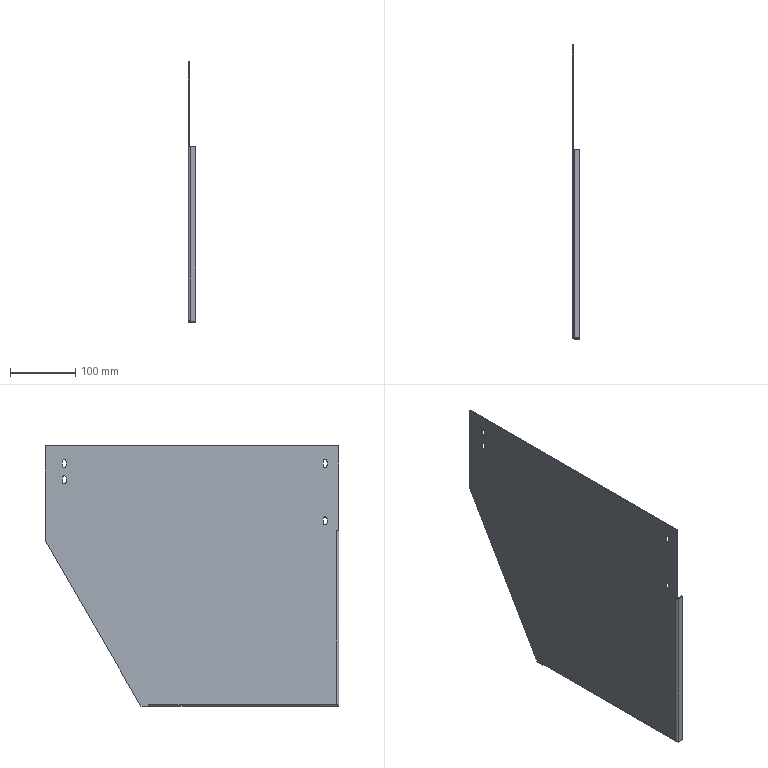Part | NX | features solid 2 | 1 solid | 50 faces | box 12 x 450 x 399 mm | volume 248985 mm3 | plane 38 | cylinder 12 | commonest cylinder face diameters 6 x10 3 x2
STEP:
#1=CARTESIAN_POINT('',(-1108.5,341.153,-601.));
#2=VERTEX_POINT('',#1);
#3=CARTESIAN_POINT('',(-1108.5,53.,-601.));
#4=VERTEX_POINT('',#3);
#5=CARTESIAN_POINT('',(-1108.5,341.153,-601.));
#6=DIRECTION('',(0.,-1.,0.));
#7=VECTOR('',#6,1000.);
#8=LINE('',#5,#7);
#9=EDGE_CURVE('',#2,#4,#8,.T.);
#10=ORIENTED_EDGE('',*,*,#9,.T.);
#11=CARTESIAN_POINT('',(-1107.,51.6,-602.5));
#12=VERTEX_POINT('',#11);
#13=CARTESIAN_POINT('',(-1107.,51.6,-602.5));
#14=CARTESIAN_POINT('',(-1107.879,51.6,-602.5));
#15=CARTESIAN_POINT('',(-1108.5,52.18,-601.879));
#16=CARTESIAN_POINT('',(-1108.5,53.,-601.));
#17=(BOUNDED_CURVE()B_SPLINE_CURVE(3,(#13,#14,#15,#16),.UNSPECIFIED.,.F.,.F.)B_SPLINE_CURVE_WITH_KNOTS((4,4),(0.,1.571),.PIECEWISE_BEZIER_KNOTS.)CURVE()GEOMETRIC_REPRESENTATION_ITEM()RATIONAL_B_SPLINE_CURVE((1.,0.8047,0.8047,1.))REPRESENTATION_ITEM(''));
#18=EDGE_CURVE('',#12,#4,#17,.T.);
#19=ORIENTED_EDGE('',*,*,#18,.F.);
#20=CARTESIAN_POINT('',(-1107.,341.153,-602.5));
#21=VERTEX_POINT('',#20);
#22=CARTESIAN_POINT('',(-1107.,53.,-602.5));
#23=DIRECTION('',(0.,1.,0.));
#24=VECTOR('',#23,1000.);
#25=LINE('',#22,#24);
#26=EDGE_CURVE('',#12,#21,#25,.T.);
#27=ORIENTED_EDGE('',*,*,#26,.T.);
#28=CARTESIAN_POINT('',(-1107.,341.153,-601.));
#29=DIRECTION('',(0.,1.,0.));
#30=DIRECTION('',(-1.,0.,0.));
#31=AXIS2_PLACEMENT_3D('',#28,#29,#30);
#32=CIRCLE('',#31,1.5);
#33=EDGE_CURVE('',#21,#2,#32,.T.);
#34=ORIENTED_EDGE('',*,*,#33,.T.);
#35=EDGE_LOOP('',(#10,#19,#27,#34));
#36=FACE_BOUND('',#35,.T.);
#37=CARTESIAN_POINT('',(-1107.,341.153,-601.));
#38=DIRECTION('',(0.,-1.,0.));
#39=DIRECTION('',(1.,0.,0.));
#40=AXIS2_PLACEMENT_3D('',#37,#38,#39);
#41=CYLINDRICAL_SURFACE('',#40,1.5);
#42=ADVANCED_FACE('',(#36),#41,.F.);
#43=CARTESIAN_POINT('',(-1110.,341.153,-601.));
#44=VERTEX_POINT('',#43);
#45=CARTESIAN_POINT('',(-1110.,53.,-601.));
#46=VERTEX_POINT('',#45);
#47=CARTESIAN_POINT('',(-1110.,341.153,-601.));
#48=DIRECTION('',(0.,-1.,0.));
#49=VECTOR('',#48,1000.);
#50=LINE('',#47,#49);
#51=EDGE_CURVE('',#44,#46,#50,.T.);
#52=ORIENTED_EDGE('',*,*,#51,.F.);
#53=CARTESIAN_POINT('',(-1107.,341.153,-604.));
#54=VERTEX_POINT('',#53);
#55=CARTESIAN_POINT('',(-1107.,341.153,-601.));
#56=DIRECTION('',(0.,1.,0.));
#57=DIRECTION('',(1.,0.,0.));
#58=AXIS2_PLACEMENT_3D('',#55,#56,#57);
#59=CIRCLE('',#58,3.);
#60=EDGE_CURVE('',#54,#44,#59,.T.);
#61=ORIENTED_EDGE('',*,*,#60,.F.);
#62=CARTESIAN_POINT('',(-1107.,51.6,-604.));
#63=VERTEX_POINT('',#62);
#64=CARTESIAN_POINT('',(-1107.,53.,-604.));
#65=DIRECTION('',(0.,1.,0.));
#66=VECTOR('',#65,1000.);
#67=LINE('',#64,#66);
#68=EDGE_CURVE('',#63,#54,#67,.T.);
#69=ORIENTED_EDGE('',*,*,#68,.F.);
#70=CARTESIAN_POINT('',(-1109.598,51.6,-602.5));
#71=VERTEX_POINT('',#70);
#72=CARTESIAN_POINT('',(-1107.,51.6,-601.));
#73=DIRECTION('',(0.,1.,0.));
#74=DIRECTION('',(1.,0.,0.));
#75=AXIS2_PLACEMENT_3D('',#72,#73,#74);
#76=CIRCLE('',#75,3.);
#77=EDGE_CURVE('',#63,#71,#76,.T.);
#78=ORIENTED_EDGE('',*,*,#77,.T.);
#79=CARTESIAN_POINT('',(-1109.598,51.6,-602.5));
#80=CARTESIAN_POINT('',(-1109.863,52.028,-602.041));
#81=CARTESIAN_POINT('',(-1110.,52.506,-601.53));
#82=CARTESIAN_POINT('',(-1110.,53.,-601.));
#83=(BOUNDED_CURVE()B_SPLINE_CURVE(3,(#79,#80,#81,#82),.UNSPECIFIED.,.F.,.F.)B_SPLINE_CURVE_WITH_KNOTS((4,4),(1.047,1.571),.PIECEWISE_BEZIER_KNOTS.)CURVE()GEOMETRIC_REPRESENTATION_ITEM()RATIONAL_B_SPLINE_CURVE((1.,0.9773,0.9773,1.))REPRESENTATION_ITEM(''));
#84=EDGE_CURVE('',#71,#46,#83,.T.);
#85=ORIENTED_EDGE('',*,*,#84,.T.);
#86=EDGE_LOOP('',(#52,#61,#69,#78,#85));
#87=FACE_BOUND('',#86,.T.);
#88=CARTESIAN_POINT('',(-1107.,341.153,-601.));
#89=DIRECTION('',(0.,-1.,0.));
#90=DIRECTION('',(1.,0.,0.));
#91=AXIS2_PLACEMENT_3D('',#88,#89,#90);
#92=CYLINDRICAL_SURFACE('',#91,3.);
#93=ADVANCED_FACE('',(#87),#92,.T.);
#94=CARTESIAN_POINT('',(-1098.,341.153,-602.5));
#95=VERTEX_POINT('',#94);
#96=CARTESIAN_POINT('',(-1098.,51.6,-602.5));
#97=VERTEX_POINT('',#96);
#98=CARTESIAN_POINT('',(-1098.,341.153,-602.5));
#99=DIRECTION('',(0.,-1.,0.));
#100=VECTOR('',#99,1000.);
#101=LINE('',#98,#100);
#102=EDGE_CURVE('',#95,#97,#101,.T.);
#103=ORIENTED_EDGE('',*,*,#102,.T.);
#104=CARTESIAN_POINT('',(-1098.,51.6,-604.));
#105=VERTEX_POINT('',#104);
#106=CARTESIAN_POINT('',(-1098.,51.6,-604.));
#107=DIRECTION('',(0.,0.,1.));
#108=VECTOR('',#107,1000.);
#109=LINE('',#106,#108);
#110=EDGE_CURVE('',#105,#97,#109,.T.);
#111=ORIENTED_EDGE('',*,*,#110,.F.);
#112=CARTESIAN_POINT('',(-1098.,341.153,-604.));
#113=VERTEX_POINT('',#112);
#114=CARTESIAN_POINT('',(-1098.,341.153,-604.));
#115=DIRECTION('',(0.,-1.,0.));
#116=VECTOR('',#115,1000.);
#117=LINE('',#114,#116);
#118=EDGE_CURVE('',#113,#105,#117,.T.);
#119=ORIENTED_EDGE('',*,*,#118,.F.);
#120=CARTESIAN_POINT('',(-1098.,341.153,-604.));
#121=DIRECTION('',(0.,0.,1.));
#122=VECTOR('',#121,1000.);
#123=LINE('',#120,#122);
#124=EDGE_CURVE('',#113,#95,#123,.T.);
#125=ORIENTED_EDGE('',*,*,#124,.T.);
#126=EDGE_LOOP('',(#103,#111,#119,#125));
#127=FACE_BOUND('',#126,.T.);
#128=CARTESIAN_POINT('',(-1098.,341.153,-604.));
#129=DIRECTION('',(-1.,0.,0.));
#130=DIRECTION('',(0.,0.,1.));
#131=AXIS2_PLACEMENT_3D('',#128,#129,#130);
#132=PLANE('',#131);
#133=ADVANCED_FACE('',(#127),#132,.F.);
#134=ORIENTED_EDGE('',*,*,#26,.F.);
#135=CARTESIAN_POINT('',(-1108.649,51.6,-602.5));
#136=DIRECTION('',(-1.,0.,0.));
#137=VECTOR('',#136,1000.);
#138=LINE('',#135,#137);
#139=EDGE_CURVE('',#97,#12,#138,.T.);
#140=ORIENTED_EDGE('',*,*,#139,.F.);
#141=ORIENTED_EDGE('',*,*,#102,.F.);
#142=CARTESIAN_POINT('',(-1108.649,341.153,-602.5));
#143=DIRECTION('',(1.,0.,0.));
#144=VECTOR('',#143,1000.);
#145=LINE('',#142,#144);
#146=EDGE_CURVE('',#21,#95,#145,.T.);
#147=ORIENTED_EDGE('',*,*,#146,.F.);
#148=EDGE_LOOP('',(#134,#140,#141,#147));
#149=FACE_BOUND('',#148,.T.);
#150=CARTESIAN_POINT('',(-722.5,275.,-602.5));
#151=DIRECTION('',(0.,0.,-1.));
#152=DIRECTION('',(-1.,0.,0.));
#153=AXIS2_PLACEMENT_3D('',#150,#151,#152);
#154=PLANE('',#153);
#155=ADVANCED_FACE('',(#149),#154,.F.);
#156=CARTESIAN_POINT('',(-1108.649,51.6,-604.));
#157=DIRECTION('',(-1.,0.,0.));
#158=VECTOR('',#157,1000.);
#159=LINE('',#156,#158);
#160=EDGE_CURVE('',#105,#63,#159,.T.);
#161=ORIENTED_EDGE('',*,*,#160,.T.);
#162=ORIENTED_EDGE('',*,*,#68,.T.);
#163=CARTESIAN_POINT('',(-1108.649,341.153,-604.));
#164=DIRECTION('',(1.,0.,0.));
#165=VECTOR('',#164,1000.);
#166=LINE('',#163,#165);
#167=EDGE_CURVE('',#54,#113,#166,.T.);
#168=ORIENTED_EDGE('',*,*,#167,.T.);
#169=ORIENTED_EDGE('',*,*,#118,.T.);
#170=EDGE_LOOP('',(#161,#162,#168,#169));
#171=FACE_BOUND('',#170,.T.);
#172=CARTESIAN_POINT('',(-722.5,275.,-604.));
#173=DIRECTION('',(0.,0.,-1.));
#174=DIRECTION('',(-1.,0.,0.));
#175=AXIS2_PLACEMENT_3D('',#172,#173,#174);
#176=PLANE('',#175);
#177=ADVANCED_FACE('',(#171),#176,.T.);
#178=CARTESIAN_POINT('',(-1107.,51.6,-604.));
#179=DIRECTION('',(0.,0.,1.));
#180=VECTOR('',#179,1000.);
#181=LINE('',#178,#180);
#182=EDGE_CURVE('',#63,#12,#181,.T.);
#183=ORIENTED_EDGE('',*,*,#182,.F.);
#184=ORIENTED_EDGE('',*,*,#160,.F.);
#185=ORIENTED_EDGE('',*,*,#110,.T.);
#186=ORIENTED_EDGE('',*,*,#139,.T.);
#187=EDGE_LOOP('',(#183,#184,#185,#186));
#188=FACE_BOUND('',#187,.T.);
#189=CARTESIAN_POINT('',(-1108.649,51.6,-604.));
#190=DIRECTION('',(0.,1.,0.));
#191=DIRECTION('',(0.,0.,-1.));
#192=AXIS2_PLACEMENT_3D('',#189,#190,#191);
#193=PLANE('',#192);
#194=ADVANCED_FACE('',(#188),#193,.F.);
#195=CARTESIAN_POINT('',(-1107.,50.,-602.4));
#196=VERTEX_POINT('',#195);
#197=CARTESIAN_POINT('',(-1107.,50.,-604.));
#198=VERTEX_POINT('',#197);
#199=CARTESIAN_POINT('',(-1107.,50.,-601.));
#200=DIRECTION('',(0.,0.,-1.));
#201=VECTOR('',#200,1000.);
#202=LINE('',#199,#201);
#203=EDGE_CURVE('',#196,#198,#202,.T.);
#204=ORIENTED_EDGE('',*,*,#203,.F.);
#205=CARTESIAN_POINT('',(-1107.,51.5,-602.4));
#206=VERTEX_POINT('',#205);
#207=CARTESIAN_POINT('',(-1107.,50.,-602.4));
#208=DIRECTION('',(0.,-1.,0.));
#209=VECTOR('',#208,1000.);
#210=LINE('',#207,#209);
#211=EDGE_CURVE('',#206,#196,#210,.T.);
#212=ORIENTED_EDGE('',*,*,#211,.F.);
#213=CARTESIAN_POINT('',(-1107.,51.5,-604.));
#214=VERTEX_POINT('',#213);
#215=CARTESIAN_POINT('',(-1107.,51.5,-601.));
#216=DIRECTION('',(0.,0.,-1.));
#217=VECTOR('',#216,1000.);
#218=LINE('',#215,#217);
#219=EDGE_CURVE('',#206,#214,#218,.T.);
#220=ORIENTED_EDGE('',*,*,#219,.T.);
#221=CARTESIAN_POINT('',(-1107.,353.353,-604.));
#222=DIRECTION('',(0.,1.,0.));
#223=VECTOR('',#222,1000.);
#224=LINE('',#221,#223);
#225=EDGE_CURVE('',#198,#214,#224,.T.);
#226=ORIENTED_EDGE('',*,*,#225,.F.);
#227=EDGE_LOOP('',(#204,#212,#220,#226));
#228=FACE_BOUND('',#227,.T.);
#229=CARTESIAN_POINT('',(-1107.,50.,-601.));
#230=DIRECTION('',(-1.,0.,0.));
#231=DIRECTION('',(0.,0.,1.));
#232=AXIS2_PLACEMENT_3D('',#229,#230,#231);
#233=PLANE('',#232);
#234=ADVANCED_FACE('',(#228),#233,.T.);
#235=CARTESIAN_POINT('',(-1108.5,341.153,-600.9));
#236=VERTEX_POINT('',#235);
#237=CARTESIAN_POINT('',(-1108.5,341.253,-600.9));
#238=VERTEX_POINT('',#237);
#239=CARTESIAN_POINT('',(-1108.5,341.153,-600.9));
#240=DIRECTION('',(0.,1.,0.));
#241=VECTOR('',#240,1000.);
#242=LINE('',#239,#241);
#243=EDGE_CURVE('',#236,#238,#242,.T.);
#244=ORIENTED_EDGE('',*,*,#243,.F.);
#245=CARTESIAN_POINT('',(-1110.,341.153,-600.9));
#246=VERTEX_POINT('',#245);
#247=CARTESIAN_POINT('',(-1110.,341.153,-600.9));
#248=DIRECTION('',(-1.,0.,0.));
#249=VECTOR('',#248,1000.);
#250=LINE('',#247,#249);
#251=EDGE_CURVE('',#236,#246,#250,.T.);
#252=ORIENTED_EDGE('',*,*,#251,.T.);
#253=CARTESIAN_POINT('',(-1110.,341.253,-600.9));
#254=VERTEX_POINT('',#253);
#255=CARTESIAN_POINT('',(-1110.,341.253,-600.9));
#256=DIRECTION('',(0.,1.,0.));
#257=VECTOR('',#256,1000.);
#258=LINE('',#255,#257);
#259=EDGE_CURVE('',#246,#254,#258,.T.);
#260=ORIENTED_EDGE('',*,*,#259,.T.);
#261=CARTESIAN_POINT('',(-1110.,341.253,-600.9));
#262=DIRECTION('',(-1.,0.,0.));
#263=VECTOR('',#262,1000.);
#264=LINE('',#261,#263);
#265=EDGE_CURVE('',#238,#254,#264,.T.);
#266=ORIENTED_EDGE('',*,*,#265,.F.);
#267=EDGE_LOOP('',(#244,#252,#260,#266));
#268=FACE_BOUND('',#267,.T.);
#269=CARTESIAN_POINT('',(-1110.,341.253,-600.9));
#270=DIRECTION('',(0.,0.,1.));
#271=DIRECTION('',(0.,-1.,0.));
#272=AXIS2_PLACEMENT_3D('',#269,#270,#271);
#273=PLANE('',#272);
#274=ADVANCED_FACE('',(#268),#273,.F.);
#275=ORIENTED_EDGE('',*,*,#265,.T.);
#276=CARTESIAN_POINT('',(-1110.,341.253,-604.));
#277=VERTEX_POINT('',#276);
#278=CARTESIAN_POINT('',(-1110.,341.253,-604.));
#279=DIRECTION('',(0.,0.,-1.));
#280=VECTOR('',#279,1000.);
#281=LINE('',#278,#280);
#282=EDGE_CURVE('',#254,#277,#281,.T.);
#283=ORIENTED_EDGE('',*,*,#282,.T.);
#284=CARTESIAN_POINT('',(-1108.5,341.253,-604.));
#285=VERTEX_POINT('',#284);
#286=CARTESIAN_POINT('',(-1110.,341.253,-604.));
#287=DIRECTION('',(-1.,0.,0.));
#288=VECTOR('',#287,1000.);
#289=LINE('',#286,#288);
#290=EDGE_CURVE('',#285,#277,#289,.T.);
#291=ORIENTED_EDGE('',*,*,#290,.F.);
#292=CARTESIAN_POINT('',(-1108.5,341.253,-600.9));
#293=DIRECTION('',(0.,0.,-1.));
#294=VECTOR('',#293,1000.);
#295=LINE('',#292,#294);
#296=EDGE_CURVE('',#238,#285,#295,.T.);
#297=ORIENTED_EDGE('',*,*,#296,.F.);
#298=EDGE_LOOP('',(#275,#283,#291,#297));
#299=FACE_BOUND('',#298,.T.);
#300=CARTESIAN_POINT('',(-1110.,341.253,-604.));
#301=DIRECTION('',(0.,1.,0.));
#302=DIRECTION('',(0.,0.,-1.));
#303=AXIS2_PLACEMENT_3D('',#300,#301,#302);
#304=PLANE('',#303);
#305=ADVANCED_FACE('',(#299),#304,.F.);
#306=CARTESIAN_POINT('',(-1110.,468.,-235.));
#307=VERTEX_POINT('',#306);
#308=CARTESIAN_POINT('',(-1108.5,468.,-235.));
#309=VERTEX_POINT('',#308);
#310=CARTESIAN_POINT('',(-1108.5,468.,-235.));
#311=DIRECTION('',(1.,0.,0.));
#312=VECTOR('',#311,1000.);
#313=LINE('',#310,#312);
#314=EDGE_CURVE('',#307,#309,#313,.T.);
#315=ORIENTED_EDGE('',*,*,#314,.T.);
#316=CARTESIAN_POINT('',(-1108.5,474.,-235.));
#317=VERTEX_POINT('',#316);
#318=CARTESIAN_POINT('',(-1108.5,471.,-235.));
#319=DIRECTION('',(-1.,0.,0.));
#320=DIRECTION('',(0.,1.,0.));
#321=AXIS2_PLACEMENT_3D('',#318,#319,#320);
#322=CIRCLE('',#321,3.);
#323=EDGE_CURVE('',#317,#309,#322,.T.);
#324=ORIENTED_EDGE('',*,*,#323,.F.);
#325=CARTESIAN_POINT('',(-1110.,474.,-235.));
#326=VERTEX_POINT('',#325);
#327=CARTESIAN_POINT('',(-1108.5,474.,-235.));
#328=DIRECTION('',(1.,0.,0.));
#329=VECTOR('',#328,1000.);
#330=LINE('',#327,#329);
#331=EDGE_CURVE('',#326,#317,#330,.T.);
#332=ORIENTED_EDGE('',*,*,#331,.F.);
#333=CARTESIAN_POINT('',(-1110.,471.,-235.));
#334=DIRECTION('',(-1.,0.,0.));
#335=DIRECTION('',(0.,1.,0.));
#336=AXIS2_PLACEMENT_3D('',#333,#334,#335);
#337=CIRCLE('',#336,3.);
#338=EDGE_CURVE('',#326,#307,#337,.T.);
#339=ORIENTED_EDGE('',*,*,#338,.T.);
#340=EDGE_LOOP('',(#315,#324,#332,#339));
#341=FACE_BOUND('',#340,.T.);
#342=CARTESIAN_POINT('',(-1108.5,471.,-235.));
#343=DIRECTION('',(-1.,0.,0.));
#344=DIRECTION('',(0.,1.,0.));
#345=AXIS2_PLACEMENT_3D('',#342,#343,#344);
#346=CYLINDRICAL_SURFACE('',#345,3.);
#347=ADVANCED_FACE('',(#341),#346,.F.);
#348=CARTESIAN_POINT('',(-1110.,468.,-229.));
#349=VERTEX_POINT('',#348);
#350=CARTESIAN_POINT('',(-1110.,474.,-229.));
#351=VERTEX_POINT('',#350);
#352=CARTESIAN_POINT('',(-1110.,471.,-229.));
#353=DIRECTION('',(-1.,0.,0.));
#354=DIRECTION('',(0.,1.,0.));
#355=AXIS2_PLACEMENT_3D('',#352,#353,#354);
#356=CIRCLE('',#355,3.);
#357=EDGE_CURVE('',#349,#351,#356,.T.);
#358=ORIENTED_EDGE('',*,*,#357,.T.);
#359=CARTESIAN_POINT('',(-1108.5,474.,-229.));
#360=VERTEX_POINT('',#359);
#361=CARTESIAN_POINT('',(-1108.5,474.,-229.));
#362=DIRECTION('',(1.,0.,0.));
#363=VECTOR('',#362,1000.);
#364=LINE('',#361,#363);
#365=EDGE_CURVE('',#351,#360,#364,.T.);
#366=ORIENTED_EDGE('',*,*,#365,.T.);
#367=CARTESIAN_POINT('',(-1108.5,468.,-229.));
#368=VERTEX_POINT('',#367);
#369=CARTESIAN_POINT('',(-1108.5,471.,-229.));
#370=DIRECTION('',(-1.,0.,0.));
#371=DIRECTION('',(0.,1.,0.));
#372=AXIS2_PLACEMENT_3D('',#369,#370,#371);
#373=CIRCLE('',#372,3.);
#374=EDGE_CURVE('',#368,#360,#373,.T.);
#375=ORIENTED_EDGE('',*,*,#374,.F.);
#376=CARTESIAN_POINT('',(-1108.5,468.,-229.));
#377=DIRECTION('',(1.,0.,0.));
#378=VECTOR('',#377,1000.);
#379=LINE('',#376,#378);
#380=EDGE_CURVE('',#349,#368,#379,.T.);
#381=ORIENTED_EDGE('',*,*,#380,.F.);
#382=EDGE_LOOP('',(#358,#366,#375,#381));
#383=FACE_BOUND('',#382,.T.);
#384=CARTESIAN_POINT('',(-1108.5,471.,-229.));
#385=DIRECTION('',(-1.,0.,0.));
#386=DIRECTION('',(0.,1.,0.));
#387=AXIS2_PLACEMENT_3D('',#384,#385,#386);
#388=CYLINDRICAL_SURFACE('',#387,3.);
#389=ADVANCED_FACE('',(#383),#388,.F.);
#390=CARTESIAN_POINT('',(-1110.,474.,-205.));
#391=DIRECTION('',(0.,0.,-1.));
#392=VECTOR('',#391,1000.);
#393=LINE('',#390,#392);
#394=EDGE_CURVE('',#351,#326,#393,.T.);
#395=ORIENTED_EDGE('',*,*,#394,.T.);
#396=ORIENTED_EDGE('',*,*,#331,.T.);
#397=CARTESIAN_POINT('',(-1108.5,474.,-205.));
#398=DIRECTION('',(0.,0.,-1.));
#399=VECTOR('',#398,1000.);
#400=LINE('',#397,#399);
#401=EDGE_CURVE('',#360,#317,#400,.T.);
#402=ORIENTED_EDGE('',*,*,#401,.F.);
#403=ORIENTED_EDGE('',*,*,#365,.F.);
#404=EDGE_LOOP('',(#395,#396,#402,#403));
#405=FACE_BOUND('',#404,.T.);
#406=CARTESIAN_POINT('',(-1108.5,474.,-205.));
#407=DIRECTION('',(0.,1.,0.));
#408=DIRECTION('',(0.,0.,-1.));
#409=AXIS2_PLACEMENT_3D('',#406,#407,#408);
#410=PLANE('',#409);
#411=ADVANCED_FACE('',(#405),#410,.F.);
#412=CARTESIAN_POINT('',(-1110.,468.,-205.));
#413=DIRECTION('',(0.,0.,1.));
#414=VECTOR('',#413,1000.);
#415=LINE('',#412,#414);
#416=EDGE_CURVE('',#307,#349,#415,.T.);
#417=ORIENTED_EDGE('',*,*,#416,.T.);
#418=ORIENTED_EDGE('',*,*,#380,.T.);
#419=CARTESIAN_POINT('',(-1108.5,468.,-205.));
#420=DIRECTION('',(0.,0.,1.));
#421=VECTOR('',#420,1000.);
#422=LINE('',#419,#421);
#423=EDGE_CURVE('',#309,#368,#422,.T.);
#424=ORIENTED_EDGE('',*,*,#423,.F.);
#425=ORIENTED_EDGE('',*,*,#314,.F.);
#426=EDGE_LOOP('',(#417,#418,#424,#425));
#427=FACE_BOUND('',#426,.T.);
#428=CARTESIAN_POINT('',(-1108.5,468.,-205.));
#429=DIRECTION('',(0.,-1.,0.));
#430=DIRECTION('',(0.,0.,-1.));
#431=AXIS2_PLACEMENT_3D('',#428,#429,#430);
#432=PLANE('',#431);
#433=ADVANCED_FACE('',(#427),#432,.F.);
#434=CARTESIAN_POINT('',(-1110.,468.,-260.));
#435=VERTEX_POINT('',#434);
#436=CARTESIAN_POINT('',(-1108.5,468.,-260.));
#437=VERTEX_POINT('',#436);
#438=CARTESIAN_POINT('',(-1108.5,468.,-260.));
#439=DIRECTION('',(1.,0.,0.));
#440=VECTOR('',#439,1000.);
#441=LINE('',#438,#440);
#442=EDGE_CURVE('',#435,#437,#441,.T.);
#443=ORIENTED_EDGE('',*,*,#442,.T.);
#444=CARTESIAN_POINT('',(-1108.5,474.,-260.));
#445=VERTEX_POINT('',#444);
#446=CARTESIAN_POINT('',(-1108.5,471.,-260.));
#447=DIRECTION('',(-1.,0.,0.));
#448=DIRECTION('',(0.,1.,0.));
#449=AXIS2_PLACEMENT_3D('',#446,#447,#448);
#450=CIRCLE('',#449,3.);
#451=EDGE_CURVE('',#445,#437,#450,.T.);
#452=ORIENTED_EDGE('',*,*,#451,.F.);
#453=CARTESIAN_POINT('',(-1110.,474.,-260.));
#454=VERTEX_POINT('',#453);
#455=CARTESIAN_POINT('',(-1108.5,474.,-260.));
#456=DIRECTION('',(1.,0.,0.));
#457=VECTOR('',#456,1000.);
#458=LINE('',#455,#457);
#459=EDGE_CURVE('',#454,#445,#458,.T.);
#460=ORIENTED_EDGE('',*,*,#459,.F.);
#461=CARTESIAN_POINT('',(-1110.,471.,-260.));
#462=DIRECTION('',(-1.,0.,0.));
#463=DIRECTION('',(0.,1.,0.));
#464=AXIS2_PLACEMENT_3D('',#461,#462,#463);
#465=CIRCLE('',#464,3.);
#466=EDGE_CURVE('',#454,#435,#465,.T.);
#467=ORIENTED_EDGE('',*,*,#466,.T.);
#468=EDGE_LOOP('',(#443,#452,#460,#467));
#469=FACE_BOUND('',#468,.T.);
#470=CARTESIAN_POINT('',(-1108.5,471.,-260.));
#471=DIRECTION('',(-1.,0.,0.));
#472=DIRECTION('',(0.,1.,0.));
#473=AXIS2_PLACEMENT_3D('',#470,#471,#472);
#474=CYLINDRICAL_SURFACE('',#473,3.);
#475=ADVANCED_FACE('',(#469),#474,.F.);
#476=CARTESIAN_POINT('',(-1110.,468.,-254.));
#477=VERTEX_POINT('',#476);
#478=CARTESIAN_POINT('',(-1110.,474.,-254.));
#479=VERTEX_POINT('',#478);
#480=CARTESIAN_POINT('',(-1110.,471.,-254.));
#481=DIRECTION('',(-1.,0.,0.));
#482=DIRECTION('',(0.,1.,0.));
#483=AXIS2_PLACEMENT_3D('',#480,#481,#482);
#484=CIRCLE('',#483,3.);
#485=EDGE_CURVE('',#477,#479,#484,.T.);
#486=ORIENTED_EDGE('',*,*,#485,.T.);
#487=CARTESIAN_POINT('',(-1108.5,474.,-254.));
#488=VERTEX_POINT('',#487);
#489=CARTESIAN_POINT('',(-1108.5,474.,-254.));
#490=DIRECTION('',(1.,0.,0.));
#491=VECTOR('',#490,1000.);
#492=LINE('',#489,#491);
#493=EDGE_CURVE('',#479,#488,#492,.T.);
#494=ORIENTED_EDGE('',*,*,#493,.T.);
#495=CARTESIAN_POINT('',(-1108.5,468.,-254.));
#496=VERTEX_POINT('',#495);
#497=CARTESIAN_POINT('',(-1108.5,471.,-254.));
#498=DIRECTION('',(-1.,0.,0.));
#499=DIRECTION('',(0.,1.,0.));
#500=AXIS2_PLACEMENT_3D('',#497,#498,#499);
#501=CIRCLE('',#500,3.);
#502=EDGE_CURVE('',#496,#488,#501,.T.);
#503=ORIENTED_EDGE('',*,*,#502,.F.);
#504=CARTESIAN_POINT('',(-1108.5,468.,-254.));
#505=DIRECTION('',(1.,0.,0.));
#506=VECTOR('',#505,1000.);
#507=LINE('',#504,#506);
#508=EDGE_CURVE('',#477,#496,#507,.T.);
#509=ORIENTED_EDGE('',*,*,#508,.F.);
#510=EDGE_LOOP('',(#486,#494,#503,#509));
#511=FACE_BOUND('',#510,.T.);
#512=CARTESIAN_POINT('',(-1108.5,471.,-254.));
#513=DIRECTION('',(-1.,0.,0.));
#514=DIRECTION('',(0.,1.,0.));
#515=AXIS2_PLACEMENT_3D('',#512,#513,#514);
#516=CYLINDRICAL_SURFACE('',#515,3.);
#517=ADVANCED_FACE('',(#511),#516,.F.);
#518=CARTESIAN_POINT('',(-1110.,474.,-205.));
#519=DIRECTION('',(0.,0.,-1.));
#520=VECTOR('',#519,1000.);
#521=LINE('',#518,#520);
#522=EDGE_CURVE('',#479,#454,#521,.T.);
#523=ORIENTED_EDGE('',*,*,#522,.T.);
#524=ORIENTED_EDGE('',*,*,#459,.T.);
#525=CARTESIAN_POINT('',(-1108.5,474.,-205.));
#526=DIRECTION('',(0.,0.,-1.));
#527=VECTOR('',#526,1000.);
#528=LINE('',#525,#527);
#529=EDGE_CURVE('',#488,#445,#528,.T.);
#530=ORIENTED_EDGE('',*,*,#529,.F.);
#531=ORIENTED_EDGE('',*,*,#493,.F.);
#532=EDGE_LOOP('',(#523,#524,#530,#531));
#533=FACE_BOUND('',#532,.T.);
#534=CARTESIAN_POINT('',(-1108.5,474.,-205.));
#535=DIRECTION('',(0.,1.,0.));
#536=DIRECTION('',(0.,0.,-1.));
#537=AXIS2_PLACEMENT_3D('',#534,#535,#536);
#538=PLANE('',#537);
#539=ADVANCED_FACE('',(#533),#538,.F.);
#540=CARTESIAN_POINT('',(-1110.,468.,-205.));
#541=DIRECTION('',(0.,0.,1.));
#542=VECTOR('',#541,1000.);
#543=LINE('',#540,#542);
#544=EDGE_CURVE('',#435,#477,#543,.T.);
#545=ORIENTED_EDGE('',*,*,#544,.T.);
#546=ORIENTED_EDGE('',*,*,#508,.T.);
#547=CARTESIAN_POINT('',(-1108.5,468.,-205.));
#548=DIRECTION('',(0.,0.,1.));
#549=VECTOR('',#548,1000.);
#550=LINE('',#547,#549);
#551=EDGE_CURVE('',#437,#496,#550,.T.);
#552=ORIENTED_EDGE('',*,*,#551,.F.);
#553=ORIENTED_EDGE('',*,*,#442,.F.);
#554=EDGE_LOOP('',(#545,#546,#552,#553));
#555=FACE_BOUND('',#554,.T.);
#556=CARTESIAN_POINT('',(-1108.5,468.,-205.));
#557=DIRECTION('',(0.,-1.,0.));
#558=DIRECTION('',(0.,0.,-1.));
#559=AXIS2_PLACEMENT_3D('',#556,#557,#558);
#560=PLANE('',#559);
#561=ADVANCED_FACE('',(#555),#560,.F.);
#562=CARTESIAN_POINT('',(-1110.,68.,-323.));
#563=VERTEX_POINT('',#562);
#564=CARTESIAN_POINT('',(-1108.5,68.,-323.));
#565=VERTEX_POINT('',#564);
#566=CARTESIAN_POINT('',(-1108.5,68.,-323.));
#567=DIRECTION('',(1.,0.,0.));
#568=VECTOR('',#567,1000.);
#569=LINE('',#566,#568);
#570=EDGE_CURVE('',#563,#565,#569,.T.);
#571=ORIENTED_EDGE('',*,*,#570,.T.);
#572=CARTESIAN_POINT('',(-1108.5,74.,-323.));
#573=VERTEX_POINT('',#572);
#574=CARTESIAN_POINT('',(-1108.5,71.,-323.));
#575=DIRECTION('',(-1.,0.,0.));
#576=DIRECTION('',(0.,1.,0.));
#577=AXIS2_PLACEMENT_3D('',#574,#575,#576);
#578=CIRCLE('',#577,3.);
#579=EDGE_CURVE('',#573,#565,#578,.T.);
#580=ORIENTED_EDGE('',*,*,#579,.F.);
#581=CARTESIAN_POINT('',(-1110.,74.,-323.));
#582=VERTEX_POINT('',#581);
#583=CARTESIAN_POINT('',(-1108.5,74.,-323.));
#584=DIRECTION('',(1.,0.,0.));
#585=VECTOR('',#584,1000.);
#586=LINE('',#583,#585);
#587=EDGE_CURVE('',#582,#573,#586,.T.);
#588=ORIENTED_EDGE('',*,*,#587,.F.);
#589=CARTESIAN_POINT('',(-1110.,71.,-323.));
#590=DIRECTION('',(-1.,0.,0.));
#591=DIRECTION('',(0.,1.,0.));
#592=AXIS2_PLACEMENT_3D('',#589,#590,#591);
#593=CIRCLE('',#592,3.);
#594=EDGE_CURVE('',#582,#563,#593,.T.);
#595=ORIENTED_EDGE('',*,*,#594,.T.);
#596=EDGE_LOOP('',(#571,#580,#588,#595));
#597=FACE_BOUND('',#596,.T.);
#598=CARTESIAN_POINT('',(-1108.5,71.,-323.));
#599=DIRECTION('',(-1.,0.,0.));
#600=DIRECTION('',(0.,1.,0.));
#601=AXIS2_PLACEMENT_3D('',#598,#599,#600);
#602=CYLINDRICAL_SURFACE('',#601,3.);
#603=ADVANCED_FACE('',(#597),#602,.F.);
#604=CARTESIAN_POINT('',(-1110.,68.,-317.));
#605=VERTEX_POINT('',#604);
#606=CARTESIAN_POINT('',(-1110.,74.,-317.));
#607=VERTEX_POINT('',#606);
#608=CARTESIAN_POINT('',(-1110.,71.,-317.));
#609=DIRECTION('',(-1.,0.,0.));
#610=DIRECTION('',(0.,1.,0.));
#611=AXIS2_PLACEMENT_3D('',#608,#609,#610);
#612=CIRCLE('',#611,3.);
#613=EDGE_CURVE('',#605,#607,#612,.T.);
#614=ORIENTED_EDGE('',*,*,#613,.T.);
#615=CARTESIAN_POINT('',(-1108.5,74.,-317.));
#616=VERTEX_POINT('',#615);
#617=CARTESIAN_POINT('',(-1108.5,74.,-317.));
#618=DIRECTION('',(1.,0.,0.));
#619=VECTOR('',#618,1000.);
#620=LINE('',#617,#619);
#621=EDGE_CURVE('',#607,#616,#620,.T.);
#622=ORIENTED_EDGE('',*,*,#621,.T.);
#623=CARTESIAN_POINT('',(-1108.5,68.,-317.));
#624=VERTEX_POINT('',#623);
#625=CARTESIAN_POINT('',(-1108.5,71.,-317.));
#626=DIRECTION('',(-1.,0.,0.));
#627=DIRECTION('',(0.,1.,0.));
#628=AXIS2_PLACEMENT_3D('',#625,#626,#627);
#629=CIRCLE('',#628,3.);
#630=EDGE_CURVE('',#624,#616,#629,.T.);
#631=ORIENTED_EDGE('',*,*,#630,.F.);
#632=CARTESIAN_POINT('',(-1108.5,68.,-317.));
#633=DIRECTION('',(1.,0.,0.));
#634=VECTOR('',#633,1000.);
#635=LINE('',#632,#634);
#636=EDGE_CURVE('',#605,#624,#635,.T.);
#637=ORIENTED_EDGE('',*,*,#636,.F.);
#638=EDGE_LOOP('',(#614,#622,#631,#637));
#639=FACE_BOUND('',#638,.T.);
#640=CARTESIAN_POINT('',(-1108.5,71.,-317.));
#641=DIRECTION('',(-1.,0.,0.));
#642=DIRECTION('',(0.,1.,0.));
#643=AXIS2_PLACEMENT_3D('',#640,#641,#642);
#644=CYLINDRICAL_SURFACE('',#643,3.);
#645=ADVANCED_FACE('',(#639),#644,.F.);
#646=CARTESIAN_POINT('',(-1110.,74.,-205.));
#647=DIRECTION('',(0.,0.,-1.));
#648=VECTOR('',#647,1000.);
#649=LINE('',#646,#648);
#650=EDGE_CURVE('',#607,#582,#649,.T.);
#651=ORIENTED_EDGE('',*,*,#650,.T.);
#652=ORIENTED_EDGE('',*,*,#587,.T.);
#653=CARTESIAN_POINT('',(-1108.5,74.,-205.));
#654=DIRECTION('',(0.,0.,-1.));
#655=VECTOR('',#654,1000.);
#656=LINE('',#653,#655);
#657=EDGE_CURVE('',#616,#573,#656,.T.);
#658=ORIENTED_EDGE('',*,*,#657,.F.);
#659=ORIENTED_EDGE('',*,*,#621,.F.);
#660=EDGE_LOOP('',(#651,#652,#658,#659));
#661=FACE_BOUND('',#660,.T.);
#662=CARTESIAN_POINT('',(-1108.5,74.,-205.));
#663=DIRECTION('',(0.,1.,0.));
#664=DIRECTION('',(0.,0.,-1.));
#665=AXIS2_PLACEMENT_3D('',#662,#663,#664);
#666=PLANE('',#665);
#667=ADVANCED_FACE('',(#661),#666,.F.);
#668=CARTESIAN_POINT('',(-1110.,68.,-205.));
#669=DIRECTION('',(0.,0.,1.));
#670=VECTOR('',#669,1000.);
#671=LINE('',#668,#670);
#672=EDGE_CURVE('',#563,#605,#671,.T.);
#673=ORIENTED_EDGE('',*,*,#672,.T.);
#674=ORIENTED_EDGE('',*,*,#636,.T.);
#675=CARTESIAN_POINT('',(-1108.5,68.,-205.));
#676=DIRECTION('',(0.,0.,1.));
#677=VECTOR('',#676,1000.);
#678=LINE('',#675,#677);
#679=EDGE_CURVE('',#565,#624,#678,.T.);
#680=ORIENTED_EDGE('',*,*,#679,.F.);
#681=ORIENTED_EDGE('',*,*,#570,.F.);
#682=EDGE_LOOP('',(#673,#674,#680,#681));
#683=FACE_BOUND('',#682,.T.);
#684=CARTESIAN_POINT('',(-1108.5,68.,-205.));
#685=DIRECTION('',(0.,-1.,0.));
#686=DIRECTION('',(0.,0.,-1.));
#687=AXIS2_PLACEMENT_3D('',#684,#685,#686);
#688=PLANE('',#687);
#689=ADVANCED_FACE('',(#683),#688,.F.);
#690=CARTESIAN_POINT('',(-1110.,68.,-235.));
#691=VERTEX_POINT('',#690);
#692=CARTESIAN_POINT('',(-1108.5,68.,-235.));
#693=VERTEX_POINT('',#692);
#694=CARTESIAN_POINT('',(-1108.5,68.,-235.));
#695=DIRECTION('',(1.,0.,0.));
#696=VECTOR('',#695,1000.);
#697=LINE('',#694,#696);
#698=EDGE_CURVE('',#691,#693,#697,.T.);
#699=ORIENTED_EDGE('',*,*,#698,.T.);
#700=CARTESIAN_POINT('',(-1108.5,74.,-235.));
#701=VERTEX_POINT('',#700);
#702=CARTESIAN_POINT('',(-1108.5,71.,-235.));
#703=DIRECTION('',(-1.,0.,0.));
#704=DIRECTION('',(0.,1.,0.));
#705=AXIS2_PLACEMENT_3D('',#702,#703,#704);
#706=CIRCLE('',#705,3.);
#707=EDGE_CURVE('',#701,#693,#706,.T.);
#708=ORIENTED_EDGE('',*,*,#707,.F.);
#709=CARTESIAN_POINT('',(-1110.,74.,-235.));
#710=VERTEX_POINT('',#709);
#711=CARTESIAN_POINT('',(-1108.5,74.,-235.));
#712=DIRECTION('',(1.,0.,0.));
#713=VECTOR('',#712,1000.);
#714=LINE('',#711,#713);
#715=EDGE_CURVE('',#710,#701,#714,.T.);
#716=ORIENTED_EDGE('',*,*,#715,.F.);
#717=CARTESIAN_POINT('',(-1110.,71.,-235.));
#718=DIRECTION('',(-1.,0.,0.));
#719=DIRECTION('',(0.,1.,0.));
#720=AXIS2_PLACEMENT_3D('',#717,#718,#719);
#721=CIRCLE('',#720,3.);
#722=EDGE_CURVE('',#710,#691,#721,.T.);
#723=ORIENTED_EDGE('',*,*,#722,.T.);
#724=EDGE_LOOP('',(#699,#708,#716,#723));
#725=FACE_BOUND('',#724,.T.);
#726=CARTESIAN_POINT('',(-1108.5,71.,-235.));
#727=DIRECTION('',(-1.,0.,0.));
#728=DIRECTION('',(0.,1.,0.));
#729=AXIS2_PLACEMENT_3D('',#726,#727,#728);
#730=CYLINDRICAL_SURFACE('',#729,3.);
#731=ADVANCED_FACE('',(#725),#730,.F.);
#732=CARTESIAN_POINT('',(-1110.,68.,-229.));
#733=VERTEX_POINT('',#732);
#734=CARTESIAN_POINT('',(-1110.,74.,-229.));
#735=VERTEX_POINT('',#734);
#736=CARTESIAN_POINT('',(-1110.,71.,-229.));
#737=DIRECTION('',(-1.,0.,0.));
#738=DIRECTION('',(0.,1.,0.));
#739=AXIS2_PLACEMENT_3D('',#736,#737,#738);
#740=CIRCLE('',#739,3.);
#741=EDGE_CURVE('',#733,#735,#740,.T.);
#742=ORIENTED_EDGE('',*,*,#741,.T.);
#743=CARTESIAN_POINT('',(-1108.5,74.,-229.));
#744=VERTEX_POINT('',#743);
#745=CARTESIAN_POINT('',(-1108.5,74.,-229.));
#746=DIRECTION('',(1.,0.,0.));
#747=VECTOR('',#746,1000.);
#748=LINE('',#745,#747);
#749=EDGE_CURVE('',#735,#744,#748,.T.);
#750=ORIENTED_EDGE('',*,*,#749,.T.);
#751=CARTESIAN_POINT('',(-1108.5,68.,-229.));
#752=VERTEX_POINT('',#751);
#753=CARTESIAN_POINT('',(-1108.5,71.,-229.));
#754=DIRECTION('',(-1.,0.,0.));
#755=DIRECTION('',(0.,1.,0.));
#756=AXIS2_PLACEMENT_3D('',#753,#754,#755);
#757=CIRCLE('',#756,3.);
#758=EDGE_CURVE('',#752,#744,#757,.T.);
#759=ORIENTED_EDGE('',*,*,#758,.F.);
#760=CARTESIAN_POINT('',(-1108.5,68.,-229.));
#761=DIRECTION('',(1.,0.,0.));
#762=VECTOR('',#761,1000.);
#763=LINE('',#760,#762);
#764=EDGE_CURVE('',#733,#752,#763,.T.);
#765=ORIENTED_EDGE('',*,*,#764,.F.);
#766=EDGE_LOOP('',(#742,#750,#759,#765));
#767=FACE_BOUND('',#766,.T.);
#768=CARTESIAN_POINT('',(-1108.5,71.,-229.));
#769=DIRECTION('',(-1.,0.,0.));
#770=DIRECTION('',(0.,1.,0.));
#771=AXIS2_PLACEMENT_3D('',#768,#769,#770);
#772=CYLINDRICAL_SURFACE('',#771,3.);
#773=ADVANCED_FACE('',(#767),#772,.F.);
#774=CARTESIAN_POINT('',(-1110.,74.,-205.));
#775=DIRECTION('',(0.,0.,-1.));
#776=VECTOR('',#775,1000.);
#777=LINE('',#774,#776);
#778=EDGE_CURVE('',#735,#710,#777,.T.);
#779=ORIENTED_EDGE('',*,*,#778,.T.);
#780=ORIENTED_EDGE('',*,*,#715,.T.);
#781=CARTESIAN_POINT('',(-1108.5,74.,-205.));
#782=DIRECTION('',(0.,0.,-1.));
#783=VECTOR('',#782,1000.);
#784=LINE('',#781,#783);
#785=EDGE_CURVE('',#744,#701,#784,.T.);
#786=ORIENTED_EDGE('',*,*,#785,.F.);
#787=ORIENTED_EDGE('',*,*,#749,.F.);
#788=EDGE_LOOP('',(#779,#780,#786,#787));
#789=FACE_BOUND('',#788,.T.);
#790=CARTESIAN_POINT('',(-1108.5,74.,-205.));
#791=DIRECTION('',(0.,1.,0.));
#792=DIRECTION('',(0.,0.,-1.));
#793=AXIS2_PLACEMENT_3D('',#790,#791,#792);
#794=PLANE('',#793);
#795=ADVANCED_FACE('',(#789),#794,.F.);
#796=CARTESIAN_POINT('',(-1110.,68.,-205.));
#797=DIRECTION('',(0.,0.,1.));
#798=VECTOR('',#797,1000.);
#799=LINE('',#796,#798);
#800=EDGE_CURVE('',#691,#733,#799,.T.);
#801=ORIENTED_EDGE('',*,*,#800,.T.);
#802=ORIENTED_EDGE('',*,*,#764,.T.);
#803=CARTESIAN_POINT('',(-1108.5,68.,-205.));
#804=DIRECTION('',(0.,0.,1.));
#805=VECTOR('',#804,1000.);
#806=LINE('',#803,#805);
#807=EDGE_CURVE('',#693,#752,#806,.T.);
#808=ORIENTED_EDGE('',*,*,#807,.F.);
#809=ORIENTED_EDGE('',*,*,#698,.F.);
#810=EDGE_LOOP('',(#801,#802,#808,#809));
#811=FACE_BOUND('',#810,.T.);
#812=CARTESIAN_POINT('',(-1108.5,68.,-205.));
#813=DIRECTION('',(0.,-1.,0.));
#814=DIRECTION('',(0.,0.,-1.));
#815=AXIS2_PLACEMENT_3D('',#812,#813,#814);
#816=PLANE('',#815);
#817=ADVANCED_FACE('',(#811),#816,.F.);
#818=CARTESIAN_POINT('',(-1107.,51.5,-335.));
#819=VERTEX_POINT('',#818);
#820=CARTESIAN_POINT('',(-1107.,51.5,-335.));
#821=DIRECTION('',(0.,0.,-1.));
#822=VECTOR('',#821,1000.);
#823=LINE('',#820,#822);
#824=EDGE_CURVE('',#819,#206,#823,.T.);
#825=ORIENTED_EDGE('',*,*,#824,.T.);
#826=CARTESIAN_POINT('',(-1107.,51.5,-602.4));
#827=CARTESIAN_POINT('',(-1107.879,51.5,-602.4));
#828=CARTESIAN_POINT('',(-1108.5,52.121,-601.82));
#829=CARTESIAN_POINT('',(-1108.5,53.,-601.));
#830=(BOUNDED_CURVE()B_SPLINE_CURVE(3,(#826,#827,#828,#829),.UNSPECIFIED.,.F.,.F.)B_SPLINE_CURVE_WITH_KNOTS((4,4),(3.142,4.712),.PIECEWISE_BEZIER_KNOTS.)CURVE()GEOMETRIC_REPRESENTATION_ITEM()RATIONAL_B_SPLINE_CURVE((1.,0.8047,0.8047,1.))REPRESENTATION_ITEM(''));
#831=EDGE_CURVE('',#206,#4,#830,.T.);
#832=ORIENTED_EDGE('',*,*,#831,.T.);
#833=CARTESIAN_POINT('',(-1108.5,53.,-335.));
#834=VERTEX_POINT('',#833);
#835=CARTESIAN_POINT('',(-1108.5,53.,-604.));
#836=DIRECTION('',(0.,0.,1.));
#837=VECTOR('',#836,1000.);
#838=LINE('',#835,#837);
#839=EDGE_CURVE('',#4,#834,#838,.T.);
#840=ORIENTED_EDGE('',*,*,#839,.T.);
#841=CARTESIAN_POINT('',(-1107.,53.,-335.));
#842=DIRECTION('',(0.,0.,-1.));
#843=DIRECTION('',(1.,0.,0.));
#844=AXIS2_PLACEMENT_3D('',#841,#842,#843);
#845=CIRCLE('',#844,1.5);
#846=EDGE_CURVE('',#819,#834,#845,.T.);
#847=ORIENTED_EDGE('',*,*,#846,.F.);
#848=EDGE_LOOP('',(#825,#832,#840,#847));
#849=FACE_BOUND('',#848,.T.);
#850=CARTESIAN_POINT('',(-1107.,53.,-604.));
#851=DIRECTION('',(0.,0.,1.));
#852=DIRECTION('',(1.,0.,0.));
#853=AXIS2_PLACEMENT_3D('',#850,#851,#852);
#854=CYLINDRICAL_SURFACE('',#853,1.5);
#855=ADVANCED_FACE('',(#849),#854,.F.);
#856=CARTESIAN_POINT('',(-1109.598,51.5,-602.4));
#857=VERTEX_POINT('',#856);
#858=CARTESIAN_POINT('',(-1107.,53.,-602.4));
#859=DIRECTION('',(0.,0.,-1.));
#860=DIRECTION('',(1.,0.,0.));
#861=AXIS2_PLACEMENT_3D('',#858,#859,#860);
#862=CIRCLE('',#861,3.);
#863=EDGE_CURVE('',#196,#857,#862,.T.);
#864=ORIENTED_EDGE('',*,*,#863,.F.);
#865=CARTESIAN_POINT('',(-1107.,50.,-335.));
#866=VERTEX_POINT('',#865);
#867=CARTESIAN_POINT('',(-1107.,50.,-335.));
#868=DIRECTION('',(0.,0.,-1.));
#869=VECTOR('',#868,1000.);
#870=LINE('',#867,#869);
#871=EDGE_CURVE('',#866,#196,#870,.T.);
#872=ORIENTED_EDGE('',*,*,#871,.F.);
#873=CARTESIAN_POINT('',(-1110.,53.,-335.));
#874=VERTEX_POINT('',#873);
#875=CARTESIAN_POINT('',(-1107.,53.,-335.));
#876=DIRECTION('',(0.,0.,-1.));
#877=DIRECTION('',(1.,0.,0.));
#878=AXIS2_PLACEMENT_3D('',#875,#876,#877);
#879=CIRCLE('',#878,3.);
#880=EDGE_CURVE('',#866,#874,#879,.T.);
#881=ORIENTED_EDGE('',*,*,#880,.T.);
#882=CARTESIAN_POINT('',(-1110.,53.,-604.));
#883=DIRECTION('',(0.,0.,1.));
#884=VECTOR('',#883,1000.);
#885=LINE('',#882,#884);
#886=EDGE_CURVE('',#46,#874,#885,.T.);
#887=ORIENTED_EDGE('',*,*,#886,.F.);
#888=CARTESIAN_POINT('',(-1109.598,51.5,-602.4));
#889=CARTESIAN_POINT('',(-1109.863,51.959,-601.972));
#890=CARTESIAN_POINT('',(-1110.,52.47,-601.494));
#891=CARTESIAN_POINT('',(-1110.,53.,-601.));
#892=(BOUNDED_CURVE()B_SPLINE_CURVE(3,(#888,#889,#890,#891),.UNSPECIFIED.,.F.,.F.)B_SPLINE_CURVE_WITH_KNOTS((4,4),(4.189,4.712),.PIECEWISE_BEZIER_KNOTS.)CURVE()GEOMETRIC_REPRESENTATION_ITEM()RATIONAL_B_SPLINE_CURVE((1.,0.9773,0.9773,1.))REPRESENTATION_ITEM(''));
#893=EDGE_CURVE('',#857,#46,#892,.T.);
#894=ORIENTED_EDGE('',*,*,#893,.F.);
#895=EDGE_LOOP('',(#864,#872,#881,#887,#894));
#896=FACE_BOUND('',#895,.T.);
#897=CARTESIAN_POINT('',(-1107.,53.,-604.));
#898=DIRECTION('',(0.,0.,1.));
#899=DIRECTION('',(1.,0.,0.));
#900=AXIS2_PLACEMENT_3D('',#897,#898,#899);
#901=CYLINDRICAL_SURFACE('',#900,3.);
#902=ADVANCED_FACE('',(#896),#901,.T.);
#903=CARTESIAN_POINT('',(-1098.,51.5,-604.));
#904=VERTEX_POINT('',#903);
#905=CARTESIAN_POINT('',(-1098.,51.5,-335.));
#906=VERTEX_POINT('',#905);
#907=CARTESIAN_POINT('',(-1098.,51.5,-604.));
#908=DIRECTION('',(0.,0.,1.));
#909=VECTOR('',#908,1000.);
#910=LINE('',#907,#909);
#911=EDGE_CURVE('',#904,#906,#910,.T.);
#912=ORIENTED_EDGE('',*,*,#911,.T.);
#913=CARTESIAN_POINT('',(-1098.,50.,-335.));
#914=VERTEX_POINT('',#913);
#915=CARTESIAN_POINT('',(-1098.,50.,-335.));
#916=DIRECTION('',(0.,1.,0.));
#917=VECTOR('',#916,1000.);
#918=LINE('',#915,#917);
#919=EDGE_CURVE('',#914,#906,#918,.T.);
#920=ORIENTED_EDGE('',*,*,#919,.F.);
#921=CARTESIAN_POINT('',(-1098.,50.,-604.));
#922=VERTEX_POINT('',#921);
#923=CARTESIAN_POINT('',(-1098.,50.,-604.));
#924=DIRECTION('',(0.,0.,1.));
#925=VECTOR('',#924,1000.);
#926=LINE('',#923,#925);
#927=EDGE_CURVE('',#922,#914,#926,.T.);
#928=ORIENTED_EDGE('',*,*,#927,.F.);
#929=CARTESIAN_POINT('',(-1098.,50.,-604.));
#930=DIRECTION('',(0.,1.,0.));
#931=VECTOR('',#930,1000.);
#932=LINE('',#929,#931);
#933=EDGE_CURVE('',#922,#904,#932,.T.);
#934=ORIENTED_EDGE('',*,*,#933,.T.);
#935=EDGE_LOOP('',(#912,#920,#928,#934));
#936=FACE_BOUND('',#935,.T.);
#937=CARTESIAN_POINT('',(-1098.,50.,-604.));
#938=DIRECTION('',(-1.,0.,0.));
#939=DIRECTION('',(0.,0.,1.));
#940=AXIS2_PLACEMENT_3D('',#937,#938,#939);
#941=PLANE('',#940);
#942=ADVANCED_FACE('',(#936),#941,.F.);
#943=ORIENTED_EDGE('',*,*,#824,.F.);
#944=CARTESIAN_POINT('',(-1098.,51.5,-335.));
#945=DIRECTION('',(-1.,0.,0.));
#946=VECTOR('',#945,1000.);
#947=LINE('',#944,#946);
#948=EDGE_CURVE('',#906,#819,#947,.T.);
#949=ORIENTED_EDGE('',*,*,#948,.F.);
#950=ORIENTED_EDGE('',*,*,#911,.F.);
#951=CARTESIAN_POINT('',(-1108.649,51.5,-604.));
#952=DIRECTION('',(1.,0.,0.));
#953=VECTOR('',#952,1000.);
#954=LINE('',#951,#953);
#955=EDGE_CURVE('',#214,#904,#954,.T.);
#956=ORIENTED_EDGE('',*,*,#955,.F.);
#957=ORIENTED_EDGE('',*,*,#219,.F.);
#958=EDGE_LOOP('',(#943,#949,#950,#956,#957));
#959=FACE_BOUND('',#958,.T.);
#960=CARTESIAN_POINT('',(-722.5,51.5,-205.));
#961=DIRECTION('',(0.,-1.,0.));
#962=DIRECTION('',(0.,0.,-1.));
#963=AXIS2_PLACEMENT_3D('',#960,#961,#962);
#964=PLANE('',#963);
#965=ADVANCED_FACE('',(#959),#964,.F.);
#966=CARTESIAN_POINT('',(-1098.,50.,-335.));
#967=DIRECTION('',(-1.,0.,0.));
#968=VECTOR('',#967,1000.);
#969=LINE('',#966,#968);
#970=EDGE_CURVE('',#914,#866,#969,.T.);
#971=ORIENTED_EDGE('',*,*,#970,.T.);
#972=ORIENTED_EDGE('',*,*,#871,.T.);
#973=ORIENTED_EDGE('',*,*,#203,.T.);
#974=CARTESIAN_POINT('',(-1108.649,50.,-604.));
#975=DIRECTION('',(1.,0.,0.));
#976=VECTOR('',#975,1000.);
#977=LINE('',#974,#976);
#978=EDGE_CURVE('',#198,#922,#977,.T.);
#979=ORIENTED_EDGE('',*,*,#978,.T.);
#980=ORIENTED_EDGE('',*,*,#927,.T.);
#981=EDGE_LOOP('',(#971,#972,#973,#979,#980));
#982=FACE_BOUND('',#981,.T.);
#983=CARTESIAN_POINT('',(-722.5,50.,-205.));
#984=DIRECTION('',(0.,-1.,0.));
#985=DIRECTION('',(0.,0.,-1.));
#986=AXIS2_PLACEMENT_3D('',#983,#984,#985);
#987=PLANE('',#986);
#988=ADVANCED_FACE('',(#982),#987,.T.);
#989=CARTESIAN_POINT('',(-1108.5,53.1,-334.9));
#990=VERTEX_POINT('',#989);
#991=CARTESIAN_POINT('',(-1110.,53.1,-334.9));
#992=VERTEX_POINT('',#991);
#993=CARTESIAN_POINT('',(-1110.,53.1,-334.9));
#994=DIRECTION('',(-1.,0.,0.));
#995=VECTOR('',#994,1000.);
#996=LINE('',#993,#995);
#997=EDGE_CURVE('',#990,#992,#996,.T.);
#998=ORIENTED_EDGE('',*,*,#997,.T.);
#999=CARTESIAN_POINT('',(-1110.,53.1,-335.));
#1000=VERTEX_POINT('',#999);
#1001=CARTESIAN_POINT('',(-1110.,53.1,-334.9));
#1002=DIRECTION('',(0.,0.,1.));
#1003=VECTOR('',#1002,1000.);
#1004=LINE('',#1001,#1003);
#1005=EDGE_CURVE('',#1000,#992,#1004,.T.);
#1006=ORIENTED_EDGE('',*,*,#1005,.F.);
#1007=CARTESIAN_POINT('',(-1108.5,53.1,-335.));
#1008=VERTEX_POINT('',#1007);
#1009=CARTESIAN_POINT('',(-1110.,53.1,-335.));
#1010=DIRECTION('',(-1.,0.,0.));
#1011=VECTOR('',#1010,1000.);
#1012=LINE('',#1009,#1011);
#1013=EDGE_CURVE('',#1008,#1000,#1012,.T.);
#1014=ORIENTED_EDGE('',*,*,#1013,.F.);
#1015=CARTESIAN_POINT('',(-1108.5,53.1,-335.));
#1016=DIRECTION('',(0.,0.,1.));
#1017=VECTOR('',#1016,1000.);
#1018=LINE('',#1015,#1017);
#1019=EDGE_CURVE('',#1008,#990,#1018,.T.);
#1020=ORIENTED_EDGE('',*,*,#1019,.T.);
#1021=EDGE_LOOP('',(#998,#1006,#1014,#1020));
#1022=FACE_BOUND('',#1021,.T.);
#1023=CARTESIAN_POINT('',(-1110.,53.1,-334.9));
#1024=DIRECTION('',(0.,1.,0.));
#1025=DIRECTION('',(0.,0.,-1.));
#1026=AXIS2_PLACEMENT_3D('',#1023,#1024,#1025);
#1027=PLANE('',#1026);
#1028=ADVANCED_FACE('',(#1022),#1027,.F.);
#1029=CARTESIAN_POINT('',(-1108.5,50.,-334.9));
#1030=VERTEX_POINT('',#1029);
#1031=CARTESIAN_POINT('',(-1110.,50.,-334.9));
#1032=VERTEX_POINT('',#1031);
#1033=CARTESIAN_POINT('',(-1110.,50.,-334.9));
#1034=DIRECTION('',(-1.,0.,0.));
#1035=VECTOR('',#1034,1000.);
#1036=LINE('',#1033,#1035);
#1037=EDGE_CURVE('',#1030,#1032,#1036,.T.);
#1038=ORIENTED_EDGE('',*,*,#1037,.T.);
#1039=CARTESIAN_POINT('',(-1110.,50.,-334.9));
#1040=DIRECTION('',(0.,-1.,0.));
#1041=VECTOR('',#1040,1000.);
#1042=LINE('',#1039,#1041);
#1043=EDGE_CURVE('',#992,#1032,#1042,.T.);
#1044=ORIENTED_EDGE('',*,*,#1043,.F.);
#1045=ORIENTED_EDGE('',*,*,#997,.F.);
#1046=CARTESIAN_POINT('',(-1108.5,53.1,-334.9));
#1047=DIRECTION('',(0.,-1.,0.));
#1048=VECTOR('',#1047,1000.);
#1049=LINE('',#1046,#1048);
#1050=EDGE_CURVE('',#990,#1030,#1049,.T.);
#1051=ORIENTED_EDGE('',*,*,#1050,.T.);
#1052=EDGE_LOOP('',(#1038,#1044,#1045,#1051));
#1053=FACE_BOUND('',#1052,.T.);
#1054=CARTESIAN_POINT('',(-1110.,50.,-334.9));
#1055=DIRECTION('',(0.,0.,1.));
#1056=DIRECTION('',(0.,-1.,0.));
#1057=AXIS2_PLACEMENT_3D('',#1054,#1055,#1056);
#1058=PLANE('',#1057);
#1059=ADVANCED_FACE('',(#1053),#1058,.F.);
#1060=ORIENTED_EDGE('',*,*,#707,.T.);
#1061=ORIENTED_EDGE('',*,*,#807,.T.);
#1062=ORIENTED_EDGE('',*,*,#758,.T.);
#1063=ORIENTED_EDGE('',*,*,#785,.T.);
#1064=EDGE_LOOP('',(#1060,#1061,#1062,#1063));
#1065=FACE_BOUND('',#1064,.T.);
#1066=ORIENTED_EDGE('',*,*,#579,.T.);
#1067=ORIENTED_EDGE('',*,*,#679,.T.);
#1068=ORIENTED_EDGE('',*,*,#630,.T.);
#1069=ORIENTED_EDGE('',*,*,#657,.T.);
#1070=EDGE_LOOP('',(#1066,#1067,#1068,#1069));
#1071=FACE_BOUND('',#1070,.T.);
#1072=ORIENTED_EDGE('',*,*,#451,.T.);
#1073=ORIENTED_EDGE('',*,*,#551,.T.);
#1074=ORIENTED_EDGE('',*,*,#502,.T.);
#1075=ORIENTED_EDGE('',*,*,#529,.T.);
#1076=EDGE_LOOP('',(#1072,#1073,#1074,#1075));
#1077=FACE_BOUND('',#1076,.T.);
#1078=ORIENTED_EDGE('',*,*,#323,.T.);
#1079=ORIENTED_EDGE('',*,*,#423,.T.);
#1080=ORIENTED_EDGE('',*,*,#374,.T.);
#1081=ORIENTED_EDGE('',*,*,#401,.T.);
#1082=EDGE_LOOP('',(#1078,#1079,#1080,#1081));
#1083=FACE_BOUND('',#1082,.T.);
#1084=ORIENTED_EDGE('',*,*,#9,.F.);
#1085=CARTESIAN_POINT('',(-1108.5,341.153,-600.9));
#1086=DIRECTION('',(0.,0.,1.));
#1087=VECTOR('',#1086,1000.);
#1088=LINE('',#1085,#1087);
#1089=EDGE_CURVE('',#2,#236,#1088,.T.);
#1090=ORIENTED_EDGE('',*,*,#1089,.T.);
#1091=ORIENTED_EDGE('',*,*,#243,.T.);
#1092=ORIENTED_EDGE('',*,*,#296,.T.);
#1093=CARTESIAN_POINT('',(-1108.5,353.353,-604.));
#1094=VERTEX_POINT('',#1093);
#1095=CARTESIAN_POINT('',(-1108.5,353.353,-604.));
#1096=DIRECTION('',(0.,-1.,0.));
#1097=VECTOR('',#1096,1000.);
#1098=LINE('',#1095,#1097);
#1099=EDGE_CURVE('',#1094,#285,#1098,.T.);
#1100=ORIENTED_EDGE('',*,*,#1099,.F.);
#1101=CARTESIAN_POINT('',(-1108.5,500.,-350.));
#1102=VERTEX_POINT('',#1101);
#1103=CARTESIAN_POINT('',(-1108.5,500.,-350.));
#1104=DIRECTION('',(0.,-0.5,-0.866));
#1105=VECTOR('',#1104,1000.);
#1106=LINE('',#1103,#1105);
#1107=EDGE_CURVE('',#1102,#1094,#1106,.T.);
#1108=ORIENTED_EDGE('',*,*,#1107,.F.);
#1109=CARTESIAN_POINT('',(-1108.5,500.,-205.));
#1110=VERTEX_POINT('',#1109);
#1111=CARTESIAN_POINT('',(-1108.5,500.,-205.));
#1112=DIRECTION('',(0.,0.,-1.));
#1113=VECTOR('',#1112,1000.);
#1114=LINE('',#1111,#1113);
#1115=EDGE_CURVE('',#1110,#1102,#1114,.T.);
#1116=ORIENTED_EDGE('',*,*,#1115,.F.);
#1117=CARTESIAN_POINT('',(-1108.5,50.,-205.));
#1118=VERTEX_POINT('',#1117);
#1119=CARTESIAN_POINT('',(-1108.5,50.,-205.));
#1120=DIRECTION('',(0.,1.,0.));
#1121=VECTOR('',#1120,1000.);
#1122=LINE('',#1119,#1121);
#1123=EDGE_CURVE('',#1118,#1110,#1122,.T.);
#1124=ORIENTED_EDGE('',*,*,#1123,.F.);
#1125=CARTESIAN_POINT('',(-1108.5,50.,-604.));
#1126=DIRECTION('',(0.,0.,1.));
#1127=VECTOR('',#1126,1000.);
#1128=LINE('',#1125,#1127);
#1129=EDGE_CURVE('',#1030,#1118,#1128,.T.);
#1130=ORIENTED_EDGE('',*,*,#1129,.F.);
#1131=ORIENTED_EDGE('',*,*,#1050,.F.);
#1132=ORIENTED_EDGE('',*,*,#1019,.F.);
#1133=CARTESIAN_POINT('',(-1108.5,53.1,-335.));
#1134=DIRECTION('',(0.,1.,0.));
#1135=VECTOR('',#1134,1000.);
#1136=LINE('',#1133,#1135);
#1137=EDGE_CURVE('',#834,#1008,#1136,.T.);
#1138=ORIENTED_EDGE('',*,*,#1137,.F.);
#1139=ORIENTED_EDGE('',*,*,#839,.F.);
#1140=EDGE_LOOP('',(#1084,#1090,#1091,#1092,#1100,#1108,#1116,#1124,#1130,#1131,#1132,#1138,#1139));
#1141=FACE_BOUND('',#1140,.T.);
#1142=CARTESIAN_POINT('',(-1108.5,275.,-205.));
#1143=DIRECTION('',(-1.,0.,0.));
#1144=DIRECTION('',(0.,0.,1.));
#1145=AXIS2_PLACEMENT_3D('',#1142,#1143,#1144);
#1146=PLANE('',#1145);
#1147=ADVANCED_FACE('',(#1065,#1071,#1077,#1083,#1141),#1146,.F.);
#1148=ORIENTED_EDGE('',*,*,#1107,.T.);
#1149=CARTESIAN_POINT('',(-1110.,353.353,-604.));
#1150=VERTEX_POINT('',#1149);
#1151=CARTESIAN_POINT('',(-1110.,353.353,-604.));
#1152=DIRECTION('',(1.,0.,0.));
#1153=VECTOR('',#1152,1000.);
#1154=LINE('',#1151,#1153);
#1155=EDGE_CURVE('',#1150,#1094,#1154,.T.);
#1156=ORIENTED_EDGE('',*,*,#1155,.F.);
#1157=CARTESIAN_POINT('',(-1110.,500.,-350.));
#1158=VERTEX_POINT('',#1157);
#1159=CARTESIAN_POINT('',(-1110.,500.,-350.));
#1160=DIRECTION('',(0.,-0.5,-0.866));
#1161=VECTOR('',#1160,1000.);
#1162=LINE('',#1159,#1161);
#1163=EDGE_CURVE('',#1158,#1150,#1162,.T.);
#1164=ORIENTED_EDGE('',*,*,#1163,.F.);
#1165=CARTESIAN_POINT('',(-1110.,500.,-350.));
#1166=DIRECTION('',(1.,0.,0.));
#1167=VECTOR('',#1166,1000.);
#1168=LINE('',#1165,#1167);
#1169=EDGE_CURVE('',#1158,#1102,#1168,.T.);
#1170=ORIENTED_EDGE('',*,*,#1169,.T.);
#1171=EDGE_LOOP('',(#1148,#1156,#1164,#1170));
#1172=FACE_BOUND('',#1171,.T.);
#1173=CARTESIAN_POINT('',(-1110.,500.,-350.));
#1174=DIRECTION('',(0.,-0.866,0.5));
#1175=DIRECTION('',(-1.,0.,0.));
#1176=AXIS2_PLACEMENT_3D('',#1173,#1174,#1175);
#1177=PLANE('',#1176);
#1178=ADVANCED_FACE('',(#1172),#1177,.F.);
#1179=ORIENTED_EDGE('',*,*,#1115,.T.);
#1180=ORIENTED_EDGE('',*,*,#1169,.F.);
#1181=CARTESIAN_POINT('',(-1110.,500.,-205.));
#1182=VERTEX_POINT('',#1181);
#1183=CARTESIAN_POINT('',(-1110.,500.,-205.));
#1184=DIRECTION('',(0.,0.,-1.));
#1185=VECTOR('',#1184,1000.);
#1186=LINE('',#1183,#1185);
#1187=EDGE_CURVE('',#1182,#1158,#1186,.T.);
#1188=ORIENTED_EDGE('',*,*,#1187,.F.);
#1189=CARTESIAN_POINT('',(-1110.,500.,-205.));
#1190=DIRECTION('',(1.,0.,0.));
#1191=VECTOR('',#1190,1000.);
#1192=LINE('',#1189,#1191);
#1193=EDGE_CURVE('',#1182,#1110,#1192,.T.);
#1194=ORIENTED_EDGE('',*,*,#1193,.T.);
#1195=EDGE_LOOP('',(#1179,#1180,#1188,#1194));
#1196=FACE_BOUND('',#1195,.T.);
#1197=CARTESIAN_POINT('',(-1110.,500.,-205.));
#1198=DIRECTION('',(0.,-1.,0.));
#1199=DIRECTION('',(-1.,0.,0.));
#1200=AXIS2_PLACEMENT_3D('',#1197,#1198,#1199);
#1201=PLANE('',#1200);
#1202=ADVANCED_FACE('',(#1196),#1201,.F.);
#1203=ORIENTED_EDGE('',*,*,#1123,.T.);
#1204=ORIENTED_EDGE('',*,*,#1193,.F.);
#1205=CARTESIAN_POINT('',(-1110.,50.,-205.));
#1206=VERTEX_POINT('',#1205);
#1207=CARTESIAN_POINT('',(-1110.,50.,-205.));
#1208=DIRECTION('',(0.,1.,0.));
#1209=VECTOR('',#1208,1000.);
#1210=LINE('',#1207,#1209);
#1211=EDGE_CURVE('',#1206,#1182,#1210,.T.);
#1212=ORIENTED_EDGE('',*,*,#1211,.F.);
#1213=CARTESIAN_POINT('',(-1110.,50.,-205.));
#1214=DIRECTION('',(1.,0.,0.));
#1215=VECTOR('',#1214,1000.);
#1216=LINE('',#1213,#1215);
#1217=EDGE_CURVE('',#1206,#1118,#1216,.T.);
#1218=ORIENTED_EDGE('',*,*,#1217,.T.);
#1219=EDGE_LOOP('',(#1203,#1204,#1212,#1218));
#1220=FACE_BOUND('',#1219,.T.);
#1221=CARTESIAN_POINT('',(-1110.,50.,-205.));
#1222=DIRECTION('',(0.,0.,-1.));
#1223=DIRECTION('',(-1.,0.,0.));
#1224=AXIS2_PLACEMENT_3D('',#1221,#1222,#1223);
#1225=PLANE('',#1224);
#1226=ADVANCED_FACE('',(#1220),#1225,.F.);
#1227=CARTESIAN_POINT('',(-1110.,50.,-604.));
#1228=DIRECTION('',(0.,0.,1.));
#1229=VECTOR('',#1228,1000.);
#1230=LINE('',#1227,#1229);
#1231=EDGE_CURVE('',#1032,#1206,#1230,.T.);
#1232=ORIENTED_EDGE('',*,*,#1231,.F.);
#1233=ORIENTED_EDGE('',*,*,#1037,.F.);
#1234=ORIENTED_EDGE('',*,*,#1129,.T.);
#1235=ORIENTED_EDGE('',*,*,#1217,.F.);
#1236=EDGE_LOOP('',(#1232,#1233,#1234,#1235));
#1237=FACE_BOUND('',#1236,.T.);
#1238=CARTESIAN_POINT('',(-1110.,50.,-604.));
#1239=DIRECTION('',(0.,1.,0.));
#1240=DIRECTION('',(0.,0.,-1.));
#1241=AXIS2_PLACEMENT_3D('',#1238,#1239,#1240);
#1242=PLANE('',#1241);
#1243=ADVANCED_FACE('',(#1237),#1242,.F.);
#1244=CARTESIAN_POINT('',(-1107.,50.,-335.));
#1245=DIRECTION('',(0.,1.,0.));
#1246=VECTOR('',#1245,1000.);
#1247=LINE('',#1244,#1246);
#1248=EDGE_CURVE('',#866,#819,#1247,.T.);
#1249=ORIENTED_EDGE('',*,*,#1248,.F.);
#1250=ORIENTED_EDGE('',*,*,#970,.F.);
#1251=ORIENTED_EDGE('',*,*,#919,.T.);
#1252=ORIENTED_EDGE('',*,*,#948,.T.);
#1253=EDGE_LOOP('',(#1249,#1250,#1251,#1252));
#1254=FACE_BOUND('',#1253,.T.);
#1255=CARTESIAN_POINT('',(-1110.,50.,-335.));
#1256=DIRECTION('',(0.,0.,-1.));
#1257=DIRECTION('',(-1.,0.,0.));
#1258=AXIS2_PLACEMENT_3D('',#1255,#1256,#1257);
#1259=PLANE('',#1258);
#1260=ADVANCED_FACE('',(#1254),#1259,.F.);
#1261=ORIENTED_EDGE('',*,*,#1099,.T.);
#1262=ORIENTED_EDGE('',*,*,#290,.T.);
#1263=CARTESIAN_POINT('',(-1110.,353.353,-604.));
#1264=DIRECTION('',(0.,-1.,0.));
#1265=VECTOR('',#1264,1000.);
#1266=LINE('',#1263,#1265);
#1267=EDGE_CURVE('',#1150,#277,#1266,.T.);
#1268=ORIENTED_EDGE('',*,*,#1267,.F.);
#1269=ORIENTED_EDGE('',*,*,#1155,.T.);
#1270=EDGE_LOOP('',(#1261,#1262,#1268,#1269));
#1271=FACE_BOUND('',#1270,.T.);
#1272=CARTESIAN_POINT('',(-1110.,353.353,-604.));
#1273=DIRECTION('',(0.,0.,1.));
#1274=DIRECTION('',(0.,-1.,0.));
#1275=AXIS2_PLACEMENT_3D('',#1272,#1273,#1274);
#1276=PLANE('',#1275);
#1277=ADVANCED_FACE('',(#1271),#1276,.F.);
#1278=ORIENTED_EDGE('',*,*,#978,.F.);
#1279=ORIENTED_EDGE('',*,*,#225,.T.);
#1280=ORIENTED_EDGE('',*,*,#955,.T.);
#1281=ORIENTED_EDGE('',*,*,#933,.F.);
#1282=EDGE_LOOP('',(#1278,#1279,#1280,#1281));
#1283=FACE_BOUND('',#1282,.T.);
#1284=CARTESIAN_POINT('',(-1110.,353.353,-604.));
#1285=DIRECTION('',(0.,0.,1.));
#1286=DIRECTION('',(0.,-1.,0.));
#1287=AXIS2_PLACEMENT_3D('',#1284,#1285,#1286);
#1288=PLANE('',#1287);
#1289=ADVANCED_FACE('',(#1283),#1288,.F.);
#1290=ORIENTED_EDGE('',*,*,#800,.F.);
#1291=ORIENTED_EDGE('',*,*,#722,.F.);
#1292=ORIENTED_EDGE('',*,*,#778,.F.);
#1293=ORIENTED_EDGE('',*,*,#741,.F.);
#1294=EDGE_LOOP('',(#1290,#1291,#1292,#1293));
#1295=FACE_BOUND('',#1294,.T.);
#1296=ORIENTED_EDGE('',*,*,#672,.F.);
#1297=ORIENTED_EDGE('',*,*,#594,.F.);
#1298=ORIENTED_EDGE('',*,*,#650,.F.);
#1299=ORIENTED_EDGE('',*,*,#613,.F.);
#1300=EDGE_LOOP('',(#1296,#1297,#1298,#1299));
#1301=FACE_BOUND('',#1300,.T.);
#1302=ORIENTED_EDGE('',*,*,#544,.F.);
#1303=ORIENTED_EDGE('',*,*,#466,.F.);
#1304=ORIENTED_EDGE('',*,*,#522,.F.);
#1305=ORIENTED_EDGE('',*,*,#485,.F.);
#1306=EDGE_LOOP('',(#1302,#1303,#1304,#1305));
#1307=FACE_BOUND('',#1306,.T.);
#1308=ORIENTED_EDGE('',*,*,#416,.F.);
#1309=ORIENTED_EDGE('',*,*,#338,.F.);
#1310=ORIENTED_EDGE('',*,*,#394,.F.);
#1311=ORIENTED_EDGE('',*,*,#357,.F.);
#1312=EDGE_LOOP('',(#1308,#1309,#1310,#1311));
#1313=FACE_BOUND('',#1312,.T.);
#1314=CARTESIAN_POINT('',(-1110.,341.153,-604.));
#1315=DIRECTION('',(0.,0.,1.));
#1316=VECTOR('',#1315,1000.);
#1317=LINE('',#1314,#1316);
#1318=EDGE_CURVE('',#44,#246,#1317,.T.);
#1319=ORIENTED_EDGE('',*,*,#1318,.F.);
#1320=ORIENTED_EDGE('',*,*,#51,.T.);
#1321=ORIENTED_EDGE('',*,*,#886,.T.);
#1322=CARTESIAN_POINT('',(-1110.,50.,-335.));
#1323=DIRECTION('',(0.,1.,0.));
#1324=VECTOR('',#1323,1000.);
#1325=LINE('',#1322,#1324);
#1326=EDGE_CURVE('',#874,#1000,#1325,.T.);
#1327=ORIENTED_EDGE('',*,*,#1326,.T.);
#1328=ORIENTED_EDGE('',*,*,#1005,.T.);
#1329=ORIENTED_EDGE('',*,*,#1043,.T.);
#1330=ORIENTED_EDGE('',*,*,#1231,.T.);
#1331=ORIENTED_EDGE('',*,*,#1211,.T.);
#1332=ORIENTED_EDGE('',*,*,#1187,.T.);
#1333=ORIENTED_EDGE('',*,*,#1163,.T.);
#1334=ORIENTED_EDGE('',*,*,#1267,.T.);
#1335=ORIENTED_EDGE('',*,*,#282,.F.);
#1336=ORIENTED_EDGE('',*,*,#259,.F.);
#1337=EDGE_LOOP('',(#1319,#1320,#1321,#1327,#1328,#1329,#1330,#1331,#1332,#1333,#1334,#1335,#1336));
#1338=FACE_BOUND('',#1337,.T.);
#1339=CARTESIAN_POINT('',(-1110.,275.,-205.));
#1340=DIRECTION('',(-1.,0.,0.));
#1341=DIRECTION('',(0.,0.,1.));
#1342=AXIS2_PLACEMENT_3D('',#1339,#1340,#1341);
#1343=PLANE('',#1342);
#1344=ADVANCED_FACE('',(#1295,#1301,#1307,#1313,#1338),#1343,.T.);
#1345=CARTESIAN_POINT('',(-1110.,341.153,-601.));
#1346=DIRECTION('',(1.,0.,0.));
#1347=VECTOR('',#1346,1000.);
#1348=LINE('',#1345,#1347);
#1349=EDGE_CURVE('',#44,#2,#1348,.T.);
#1350=ORIENTED_EDGE('',*,*,#1349,.F.);
#1351=ORIENTED_EDGE('',*,*,#1318,.T.);
#1352=ORIENTED_EDGE('',*,*,#251,.F.);
#1353=ORIENTED_EDGE('',*,*,#1089,.F.);
#1354=EDGE_LOOP('',(#1350,#1351,#1352,#1353));
#1355=FACE_BOUND('',#1354,.T.);
#1356=CARTESIAN_POINT('',(-1110.,341.153,-604.));
#1357=DIRECTION('',(0.,-1.,0.));
#1358=DIRECTION('',(0.,0.,-1.));
#1359=AXIS2_PLACEMENT_3D('',#1356,#1357,#1358);
#1360=PLANE('',#1359);
#1361=ADVANCED_FACE('',(#1355),#1360,.F.);
#1362=CARTESIAN_POINT('',(-1107.,51.5,-602.4));
#1363=DIRECTION('',(1.,0.,0.));
#1364=VECTOR('',#1363,1000.);
#1365=LINE('',#1362,#1364);
#1366=EDGE_CURVE('',#857,#206,#1365,.T.);
#1367=ORIENTED_EDGE('',*,*,#1366,.F.);
#1368=ORIENTED_EDGE('',*,*,#893,.T.);
#1369=CARTESIAN_POINT('',(-1110.,53.,-601.));
#1370=DIRECTION('',(-1.,0.,0.));
#1371=VECTOR('',#1370,1000.);
#1372=LINE('',#1369,#1371);
#1373=EDGE_CURVE('',#4,#46,#1372,.T.);
#1374=ORIENTED_EDGE('',*,*,#1373,.F.);
#1375=ORIENTED_EDGE('',*,*,#831,.F.);
#1376=EDGE_LOOP('',(#1367,#1368,#1374,#1375));
#1377=FACE_BOUND('',#1376,.T.);
#1378=CARTESIAN_POINT('',(-1107.,53.,-601.));
#1379=DIRECTION('',(0.,-0.6823,0.7311));
#1380=DIRECTION('',(-1.,0.,0.));
#1381=AXIS2_PLACEMENT_3D('',#1378,#1379,#1380);
#1382=PLANE('',#1381);
#1383=ADVANCED_FACE('',(#1377),#1382,.F.);
#1384=CARTESIAN_POINT('',(-1110.,53.,-335.));
#1385=DIRECTION('',(1.,0.,0.));
#1386=VECTOR('',#1385,1000.);
#1387=LINE('',#1384,#1386);
#1388=EDGE_CURVE('',#874,#834,#1387,.T.);
#1389=ORIENTED_EDGE('',*,*,#1388,.F.);
#1390=ORIENTED_EDGE('',*,*,#880,.F.);
#1391=ORIENTED_EDGE('',*,*,#1248,.T.);
#1392=ORIENTED_EDGE('',*,*,#846,.T.);
#1393=EDGE_LOOP('',(#1389,#1390,#1391,#1392));
#1394=FACE_BOUND('',#1393,.T.);
#1395=CARTESIAN_POINT('',(-1110.,50.,-335.));
#1396=DIRECTION('',(0.,0.,-1.));
#1397=DIRECTION('',(-1.,0.,0.));
#1398=AXIS2_PLACEMENT_3D('',#1395,#1396,#1397);
#1399=PLANE('',#1398);
#1400=ADVANCED_FACE('',(#1394),#1399,.F.);
#1401=ORIENTED_EDGE('',*,*,#1326,.F.);
#1402=ORIENTED_EDGE('',*,*,#1388,.T.);
#1403=ORIENTED_EDGE('',*,*,#1137,.T.);
#1404=ORIENTED_EDGE('',*,*,#1013,.T.);
#1405=EDGE_LOOP('',(#1401,#1402,#1403,#1404));
#1406=FACE_BOUND('',#1405,.T.);
#1407=CARTESIAN_POINT('',(-1110.,50.,-335.));
#1408=DIRECTION('',(0.,0.,-1.));
#1409=DIRECTION('',(-1.,0.,0.));
#1410=AXIS2_PLACEMENT_3D('',#1407,#1408,#1409);
#1411=PLANE('',#1410);
#1412=ADVANCED_FACE('',(#1406),#1411,.F.);
#1413=CARTESIAN_POINT('',(-1107.,341.153,-604.));
#1414=DIRECTION('',(0.,0.,1.));
#1415=VECTOR('',#1414,1000.);
#1416=LINE('',#1413,#1415);
#1417=EDGE_CURVE('',#54,#21,#1416,.T.);
#1418=ORIENTED_EDGE('',*,*,#1417,.F.);
#1419=ORIENTED_EDGE('',*,*,#60,.T.);
#1420=ORIENTED_EDGE('',*,*,#1349,.T.);
#1421=ORIENTED_EDGE('',*,*,#33,.F.);
#1422=EDGE_LOOP('',(#1418,#1419,#1420,#1421));
#1423=FACE_BOUND('',#1422,.T.);
#1424=CARTESIAN_POINT('',(-1110.,341.153,-604.));
#1425=DIRECTION('',(0.,-1.,0.));
#1426=DIRECTION('',(0.,0.,-1.));
#1427=AXIS2_PLACEMENT_3D('',#1424,#1425,#1426);
#1428=PLANE('',#1427);
#1429=ADVANCED_FACE('',(#1423),#1428,.F.);
#1430=CARTESIAN_POINT('',(-1108.649,51.6,-602.5));
#1431=DIRECTION('',(1.,0.,0.));
#1432=VECTOR('',#1431,1000.);
#1433=LINE('',#1430,#1432);
#1434=EDGE_CURVE('',#71,#12,#1433,.T.);
#1435=ORIENTED_EDGE('',*,*,#1434,.F.);
#1436=ORIENTED_EDGE('',*,*,#77,.F.);
#1437=ORIENTED_EDGE('',*,*,#182,.T.);
#1438=EDGE_LOOP('',(#1435,#1436,#1437));
#1439=FACE_BOUND('',#1438,.T.);
#1440=CARTESIAN_POINT('',(-1108.649,51.6,-604.));
#1441=DIRECTION('',(0.,1.,0.));
#1442=DIRECTION('',(0.,0.,-1.));
#1443=AXIS2_PLACEMENT_3D('',#1440,#1441,#1442);
#1444=PLANE('',#1443);
#1445=ADVANCED_FACE('',(#1439),#1444,.F.);
#1446=ORIENTED_EDGE('',*,*,#167,.F.);
#1447=ORIENTED_EDGE('',*,*,#1417,.T.);
#1448=ORIENTED_EDGE('',*,*,#146,.T.);
#1449=ORIENTED_EDGE('',*,*,#124,.F.);
#1450=EDGE_LOOP('',(#1446,#1447,#1448,#1449));
#1451=FACE_BOUND('',#1450,.T.);
#1452=CARTESIAN_POINT('',(-1110.,341.153,-604.));
#1453=DIRECTION('',(0.,-1.,0.));
#1454=DIRECTION('',(0.,0.,-1.));
#1455=AXIS2_PLACEMENT_3D('',#1452,#1453,#1454);
#1456=PLANE('',#1455);
#1457=ADVANCED_FACE('',(#1451),#1456,.F.);
#1458=ORIENTED_EDGE('',*,*,#863,.T.);
#1459=ORIENTED_EDGE('',*,*,#1366,.T.);
#1460=ORIENTED_EDGE('',*,*,#211,.T.);
#1461=EDGE_LOOP('',(#1458,#1459,#1460));
#1462=FACE_BOUND('',#1461,.T.);
#1463=CARTESIAN_POINT('',(-1107.,53.,-602.4));
#1464=DIRECTION('',(0.,0.,1.));
#1465=DIRECTION('',(0.,-1.,0.));
#1466=AXIS2_PLACEMENT_3D('',#1463,#1464,#1465);
#1467=PLANE('',#1466);
#1468=ADVANCED_FACE('',(#1462),#1467,.F.);
#1469=ORIENTED_EDGE('',*,*,#84,.F.);
#1470=ORIENTED_EDGE('',*,*,#1434,.T.);
#1471=ORIENTED_EDGE('',*,*,#18,.T.);
#1472=ORIENTED_EDGE('',*,*,#1373,.T.);
#1473=EDGE_LOOP('',(#1469,#1470,#1471,#1472));
#1474=FACE_BOUND('',#1473,.T.);
#1475=CARTESIAN_POINT('',(-1108.649,50.953,-603.193));
#1476=DIRECTION('',(0.,0.7311,-0.6823));
#1477=DIRECTION('',(-1.,0.,0.));
#1478=AXIS2_PLACEMENT_3D('',#1475,#1476,#1477);
#1479=PLANE('',#1478);
#1480=ADVANCED_FACE('',(#1474),#1479,.F.);
#1481=CLOSED_SHELL('',(#42,#93,#133,#155,#177,#194,#234,#274,#305,#347,#389,#411,#433,#475,#517,#539,#561,#603,#645,#667,#689,#731,#773,#795,#817,#855,#902,#942,#965,#988,#1028,#1059,#1147,#1178,#1202,#1226,#1243,#1260,#1277,#1289,#1344,#1361,#1383,#1400,#1412,#1429,#1445,#1457,#1468,#1480));
#1482=MANIFOLD_SOLID_BREP('',#1481);
#1483=(LENGTH_UNIT()NAMED_UNIT(*)SI_UNIT(.MILLI.,.METRE.));
#1484=UNCERTAINTY_MEASURE_WITH_UNIT(LENGTH_MEASURE(0.00001),#1483,'','');
#1485=(NAMED_UNIT(*)PLANE_ANGLE_UNIT()SI_UNIT($,.RADIAN.));
#1486=(NAMED_UNIT(*)SI_UNIT($,.STERADIAN.)SOLID_ANGLE_UNIT());
#1487=(GEOMETRIC_REPRESENTATION_CONTEXT(3)GLOBAL_UNCERTAINTY_ASSIGNED_CONTEXT((#1484))GLOBAL_UNIT_ASSIGNED_CONTEXT((#1483,#1485,#1486))REPRESENTATION_CONTEXT('',''));
#1488=ADVANCED_BREP_SHAPE_REPRESENTATION('',(#1482),#1487);